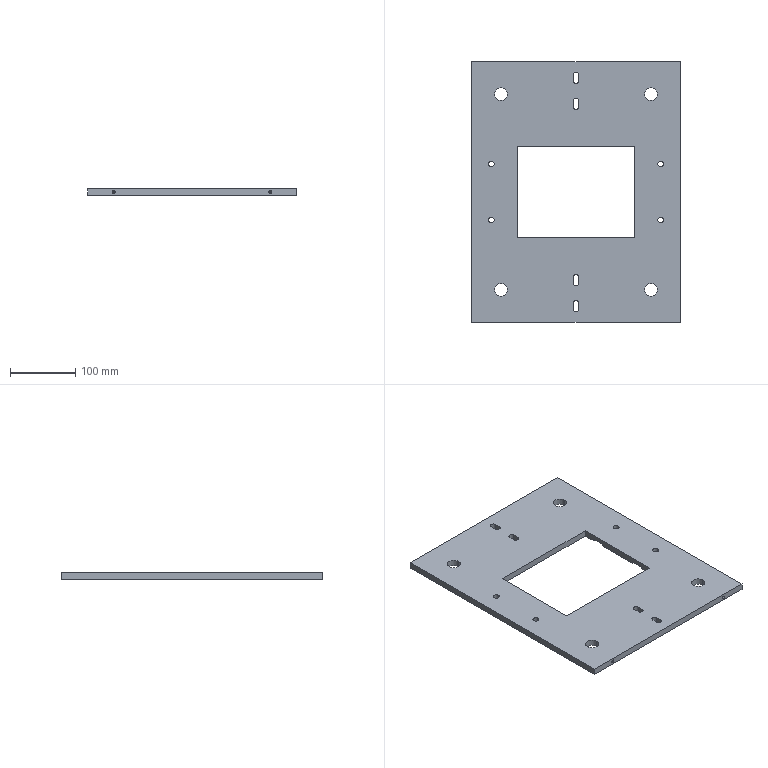Part | STEP file | 44-02-21 Press-fit Locating Plate | 1 solid | 90 faces | box 320 x 400 x 10 mm | volume 995471 mm3 | cylinder 44 | plane 34 | cone 12 | commonest cylinder face diameters 9 x16 4.2 x12 10 x8 20 x8